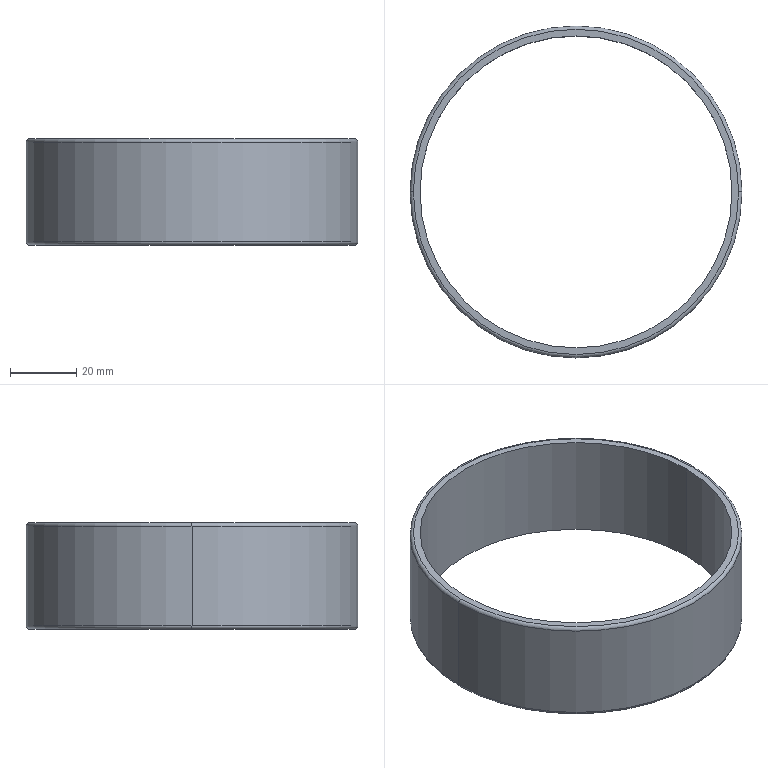Part | SolidWorks | features Extrusion 1, Fillet 1 | 1 solid | 10 faces | box 100 x 100 x 32 mm | volume 29120 mm3 | torus 4 | cylinder 4 | plane 2 | commonest cylinder face diameters 94 x2 100 x2
STEP:
#1=CARTESIAN_POINT('',(-50.,0.,31.));
#2=VERTEX_POINT('',#1);
#3=CARTESIAN_POINT('',(50.,0.,31.));
#4=VERTEX_POINT('',#3);
#5=CARTESIAN_POINT('',(0.,0.,31.));
#6=DIRECTION('',(0.,0.,-1.));
#7=DIRECTION('',(1.,0.,0.));
#8=AXIS2_PLACEMENT_3D('',#5,#6,#7);
#9=CIRCLE('',#8,50.);
#10=EDGE_CURVE('',#2,#4,#9,.T.);
#11=ORIENTED_EDGE('',*,*,#10,.F.);
#12=CARTESIAN_POINT('',(-49.,0.,32.));
#13=VERTEX_POINT('',#12);
#14=CARTESIAN_POINT('',(-49.,0.,31.));
#15=DIRECTION('',(0.,1.,0.));
#16=DIRECTION('',(-1.,0.,0.));
#17=AXIS2_PLACEMENT_3D('',#14,#15,#16);
#18=CIRCLE('',#17,1.);
#19=EDGE_CURVE('',#2,#13,#18,.T.);
#20=ORIENTED_EDGE('',*,*,#19,.T.);
#21=CARTESIAN_POINT('',(49.,0.,32.));
#22=VERTEX_POINT('',#21);
#23=CARTESIAN_POINT('',(0.,0.,32.));
#24=DIRECTION('',(0.,0.,1.));
#25=DIRECTION('',(1.,0.,0.));
#26=AXIS2_PLACEMENT_3D('',#23,#24,#25);
#27=CIRCLE('',#26,49.);
#28=EDGE_CURVE('',#22,#13,#27,.T.);
#29=ORIENTED_EDGE('',*,*,#28,.F.);
#30=CARTESIAN_POINT('',(49.,0.,31.));
#31=DIRECTION('',(0.,-1.,0.));
#32=DIRECTION('',(0.,0.,-1.));
#33=AXIS2_PLACEMENT_3D('',#30,#31,#32);
#34=CIRCLE('',#33,1.);
#35=EDGE_CURVE('',#4,#22,#34,.T.);
#36=ORIENTED_EDGE('',*,*,#35,.F.);
#37=EDGE_LOOP('',(#11,#20,#29,#36));
#38=FACE_OUTER_BOUND('',#37,.T.);
#39=CARTESIAN_POINT('',(0.,0.,31.));
#40=DIRECTION('',(0.,0.,1.));
#41=DIRECTION('',(1.,0.,0.));
#42=AXIS2_PLACEMENT_3D('',#39,#40,#41);
#43=TOROIDAL_SURFACE('',#42,49.,1.);
#44=ADVANCED_FACE('',(#38),#43,.T.);
#45=CARTESIAN_POINT('',(-49.,0.,0.));
#46=VERTEX_POINT('',#45);
#47=CARTESIAN_POINT('',(49.,0.,0.));
#48=VERTEX_POINT('',#47);
#49=CARTESIAN_POINT('',(0.,0.,0.));
#50=DIRECTION('',(0.,0.,-1.));
#51=DIRECTION('',(1.,0.,0.));
#52=AXIS2_PLACEMENT_3D('',#49,#50,#51);
#53=CIRCLE('',#52,49.);
#54=EDGE_CURVE('',#46,#48,#53,.T.);
#55=ORIENTED_EDGE('',*,*,#54,.F.);
#56=CARTESIAN_POINT('',(-50.,0.,1.));
#57=VERTEX_POINT('',#56);
#58=CARTESIAN_POINT('',(-49.,0.,1.));
#59=DIRECTION('',(0.,1.,0.));
#60=DIRECTION('',(-1.,0.,0.));
#61=AXIS2_PLACEMENT_3D('',#58,#59,#60);
#62=CIRCLE('',#61,1.);
#63=EDGE_CURVE('',#46,#57,#62,.T.);
#64=ORIENTED_EDGE('',*,*,#63,.T.);
#65=CARTESIAN_POINT('',(50.,0.,1.));
#66=VERTEX_POINT('',#65);
#67=CARTESIAN_POINT('',(0.,0.,1.));
#68=DIRECTION('',(0.,0.,1.));
#69=DIRECTION('',(1.,0.,0.));
#70=AXIS2_PLACEMENT_3D('',#67,#68,#69);
#71=CIRCLE('',#70,50.);
#72=EDGE_CURVE('',#66,#57,#71,.T.);
#73=ORIENTED_EDGE('',*,*,#72,.F.);
#74=CARTESIAN_POINT('',(49.,0.,1.));
#75=DIRECTION('',(0.,-1.,0.));
#76=DIRECTION('',(0.,0.,-1.));
#77=AXIS2_PLACEMENT_3D('',#74,#75,#76);
#78=CIRCLE('',#77,1.);
#79=EDGE_CURVE('',#48,#66,#78,.T.);
#80=ORIENTED_EDGE('',*,*,#79,.F.);
#81=EDGE_LOOP('',(#55,#64,#73,#80));
#82=FACE_OUTER_BOUND('',#81,.T.);
#83=CARTESIAN_POINT('',(0.,0.,1.));
#84=DIRECTION('',(0.,0.,1.));
#85=DIRECTION('',(1.,0.,0.));
#86=AXIS2_PLACEMENT_3D('',#83,#84,#85);
#87=TOROIDAL_SURFACE('',#86,49.,1.);
#88=ADVANCED_FACE('',(#82),#87,.T.);
#89=CARTESIAN_POINT('',(-47.,0.,32.));
#90=VERTEX_POINT('',#89);
#91=CARTESIAN_POINT('',(47.,0.,32.));
#92=VERTEX_POINT('',#91);
#93=CARTESIAN_POINT('',(0.,0.,32.));
#94=DIRECTION('',(0.,0.,1.));
#95=DIRECTION('',(1.,0.,0.));
#96=AXIS2_PLACEMENT_3D('',#93,#94,#95);
#97=CIRCLE('',#96,47.);
#98=EDGE_CURVE('',#90,#92,#97,.T.);
#99=ORIENTED_EDGE('',*,*,#98,.T.);
#100=CARTESIAN_POINT('',(47.,0.,0.));
#101=VERTEX_POINT('',#100);
#102=CARTESIAN_POINT('',(47.,0.,32.));
#103=DIRECTION('',(0.,0.,-1.));
#104=VECTOR('',#103,1000.);
#105=LINE('',#102,#104);
#106=EDGE_CURVE('',#92,#101,#105,.T.);
#107=ORIENTED_EDGE('',*,*,#106,.T.);
#108=CARTESIAN_POINT('',(-47.,0.,0.));
#109=VERTEX_POINT('',#108);
#110=CARTESIAN_POINT('',(0.,0.,0.));
#111=DIRECTION('',(0.,0.,1.));
#112=DIRECTION('',(1.,0.,0.));
#113=AXIS2_PLACEMENT_3D('',#110,#111,#112);
#114=CIRCLE('',#113,47.);
#115=EDGE_CURVE('',#109,#101,#114,.T.);
#116=ORIENTED_EDGE('',*,*,#115,.F.);
#117=CARTESIAN_POINT('',(-47.,0.,32.));
#118=DIRECTION('',(0.,0.,-1.));
#119=VECTOR('',#118,1000.);
#120=LINE('',#117,#119);
#121=EDGE_CURVE('',#90,#109,#120,.T.);
#122=ORIENTED_EDGE('',*,*,#121,.F.);
#123=EDGE_LOOP('',(#99,#107,#116,#122));
#124=FACE_OUTER_BOUND('',#123,.T.);
#125=CARTESIAN_POINT('',(0.,0.,32.));
#126=DIRECTION('',(0.,0.,-1.));
#127=DIRECTION('',(-1.,0.,0.));
#128=AXIS2_PLACEMENT_3D('',#125,#126,#127);
#129=CYLINDRICAL_SURFACE('',#128,47.);
#130=ADVANCED_FACE('',(#124),#129,.F.);
#131=ORIENTED_EDGE('',*,*,#10,.T.);
#132=CARTESIAN_POINT('',(50.,0.,32.));
#133=DIRECTION('',(0.,0.,-1.));
#134=VECTOR('',#133,1000.);
#135=LINE('',#132,#134);
#136=EDGE_CURVE('',#4,#66,#135,.T.);
#137=ORIENTED_EDGE('',*,*,#136,.T.);
#138=ORIENTED_EDGE('',*,*,#72,.T.);
#139=CARTESIAN_POINT('',(-50.,0.,32.));
#140=DIRECTION('',(0.,0.,-1.));
#141=VECTOR('',#140,1000.);
#142=LINE('',#139,#141);
#143=EDGE_CURVE('',#2,#57,#142,.T.);
#144=ORIENTED_EDGE('',*,*,#143,.F.);
#145=EDGE_LOOP('',(#131,#137,#138,#144));
#146=FACE_OUTER_BOUND('',#145,.T.);
#147=CARTESIAN_POINT('',(0.,0.,32.));
#148=DIRECTION('',(0.,0.,-1.));
#149=DIRECTION('',(-1.,0.,0.));
#150=AXIS2_PLACEMENT_3D('',#147,#148,#149);
#151=CYLINDRICAL_SURFACE('',#150,50.);
#152=ADVANCED_FACE('',(#146),#151,.T.);
#153=ORIENTED_EDGE('',*,*,#28,.T.);
#154=CARTESIAN_POINT('',(0.,0.,32.));
#155=DIRECTION('',(0.,0.,1.));
#156=DIRECTION('',(1.,0.,0.));
#157=AXIS2_PLACEMENT_3D('',#154,#155,#156);
#158=CIRCLE('',#157,49.);
#159=EDGE_CURVE('',#13,#22,#158,.T.);
#160=ORIENTED_EDGE('',*,*,#159,.T.);
#161=EDGE_LOOP('',(#153,#160));
#162=FACE_OUTER_BOUND('',#161,.T.);
#163=ORIENTED_EDGE('',*,*,#98,.F.);
#164=CARTESIAN_POINT('',(0.,0.,32.));
#165=DIRECTION('',(0.,0.,1.));
#166=DIRECTION('',(1.,0.,0.));
#167=AXIS2_PLACEMENT_3D('',#164,#165,#166);
#168=CIRCLE('',#167,47.);
#169=EDGE_CURVE('',#92,#90,#168,.T.);
#170=ORIENTED_EDGE('',*,*,#169,.F.);
#171=EDGE_LOOP('',(#163,#170));
#172=FACE_BOUND('',#171,.T.);
#173=CARTESIAN_POINT('',(0.,0.,32.));
#174=DIRECTION('',(0.,0.,1.));
#175=DIRECTION('',(1.,0.,0.));
#176=AXIS2_PLACEMENT_3D('',#173,#174,#175);
#177=PLANE('',#176);
#178=ADVANCED_FACE('',(#162,#172),#177,.T.);
#179=CARTESIAN_POINT('',(0.,0.,0.));
#180=DIRECTION('',(0.,0.,-1.));
#181=DIRECTION('',(1.,0.,0.));
#182=AXIS2_PLACEMENT_3D('',#179,#180,#181);
#183=CIRCLE('',#182,49.);
#184=EDGE_CURVE('',#48,#46,#183,.T.);
#185=ORIENTED_EDGE('',*,*,#184,.T.);
#186=ORIENTED_EDGE('',*,*,#54,.T.);
#187=EDGE_LOOP('',(#185,#186));
#188=FACE_OUTER_BOUND('',#187,.T.);
#189=ORIENTED_EDGE('',*,*,#115,.T.);
#190=CARTESIAN_POINT('',(0.,0.,0.));
#191=DIRECTION('',(0.,0.,1.));
#192=DIRECTION('',(1.,0.,0.));
#193=AXIS2_PLACEMENT_3D('',#190,#191,#192);
#194=CIRCLE('',#193,47.);
#195=EDGE_CURVE('',#101,#109,#194,.T.);
#196=ORIENTED_EDGE('',*,*,#195,.T.);
#197=EDGE_LOOP('',(#189,#196));
#198=FACE_BOUND('',#197,.T.);
#199=CARTESIAN_POINT('',(0.,0.,0.));
#200=DIRECTION('',(0.,0.,1.));
#201=DIRECTION('',(1.,0.,0.));
#202=AXIS2_PLACEMENT_3D('',#199,#200,#201);
#203=PLANE('',#202);
#204=ADVANCED_FACE('',(#188,#198),#203,.F.);
#205=ORIENTED_EDGE('',*,*,#136,.F.);
#206=CARTESIAN_POINT('',(0.,0.,31.));
#207=DIRECTION('',(0.,0.,-1.));
#208=DIRECTION('',(1.,0.,0.));
#209=AXIS2_PLACEMENT_3D('',#206,#207,#208);
#210=CIRCLE('',#209,50.);
#211=EDGE_CURVE('',#4,#2,#210,.T.);
#212=ORIENTED_EDGE('',*,*,#211,.T.);
#213=ORIENTED_EDGE('',*,*,#143,.T.);
#214=CARTESIAN_POINT('',(0.,0.,1.));
#215=DIRECTION('',(0.,0.,1.));
#216=DIRECTION('',(1.,0.,0.));
#217=AXIS2_PLACEMENT_3D('',#214,#215,#216);
#218=CIRCLE('',#217,50.);
#219=EDGE_CURVE('',#57,#66,#218,.T.);
#220=ORIENTED_EDGE('',*,*,#219,.T.);
#221=EDGE_LOOP('',(#205,#212,#213,#220));
#222=FACE_OUTER_BOUND('',#221,.T.);
#223=CARTESIAN_POINT('',(0.,0.,32.));
#224=DIRECTION('',(0.,0.,-1.));
#225=DIRECTION('',(-1.,0.,0.));
#226=AXIS2_PLACEMENT_3D('',#223,#224,#225);
#227=CYLINDRICAL_SURFACE('',#226,50.);
#228=ADVANCED_FACE('',(#222),#227,.T.);
#229=ORIENTED_EDGE('',*,*,#106,.F.);
#230=ORIENTED_EDGE('',*,*,#169,.T.);
#231=ORIENTED_EDGE('',*,*,#121,.T.);
#232=ORIENTED_EDGE('',*,*,#195,.F.);
#233=EDGE_LOOP('',(#229,#230,#231,#232));
#234=FACE_OUTER_BOUND('',#233,.T.);
#235=CARTESIAN_POINT('',(0.,0.,32.));
#236=DIRECTION('',(0.,0.,-1.));
#237=DIRECTION('',(-1.,0.,0.));
#238=AXIS2_PLACEMENT_3D('',#235,#236,#237);
#239=CYLINDRICAL_SURFACE('',#238,47.);
#240=ADVANCED_FACE('',(#234),#239,.F.);
#241=ORIENTED_EDGE('',*,*,#63,.F.);
#242=ORIENTED_EDGE('',*,*,#184,.F.);
#243=ORIENTED_EDGE('',*,*,#79,.T.);
#244=ORIENTED_EDGE('',*,*,#219,.F.);
#245=EDGE_LOOP('',(#241,#242,#243,#244));
#246=FACE_OUTER_BOUND('',#245,.T.);
#247=CARTESIAN_POINT('',(0.,0.,1.));
#248=DIRECTION('',(0.,0.,1.));
#249=DIRECTION('',(1.,0.,0.));
#250=AXIS2_PLACEMENT_3D('',#247,#248,#249);
#251=TOROIDAL_SURFACE('',#250,49.,1.);
#252=ADVANCED_FACE('',(#246),#251,.T.);
#253=ORIENTED_EDGE('',*,*,#19,.F.);
#254=ORIENTED_EDGE('',*,*,#211,.F.);
#255=ORIENTED_EDGE('',*,*,#35,.T.);
#256=ORIENTED_EDGE('',*,*,#159,.F.);
#257=EDGE_LOOP('',(#253,#254,#255,#256));
#258=FACE_OUTER_BOUND('',#257,.T.);
#259=CARTESIAN_POINT('',(0.,0.,31.));
#260=DIRECTION('',(0.,0.,1.));
#261=DIRECTION('',(1.,0.,0.));
#262=AXIS2_PLACEMENT_3D('',#259,#260,#261);
#263=TOROIDAL_SURFACE('',#262,49.,1.);
#264=ADVANCED_FACE('',(#258),#263,.T.);
#265=CLOSED_SHELL('',(#44,#88,#130,#152,#178,#204,#228,#240,#252,#264));
#266=MANIFOLD_SOLID_BREP('',#265);
#267=CARTESIAN_POINT('',(0.,0.,0.));
#268=DIRECTION('',(0.,0.,1.));
#269=DIRECTION('',(1.,0.,0.));
#270=AXIS2_PLACEMENT_3D('',#267,#268,#269);
#271=(LENGTH_UNIT()NAMED_UNIT(*)SI_UNIT(.MILLI.,.METRE.));
#272=UNCERTAINTY_MEASURE_WITH_UNIT(LENGTH_MEASURE(0.00001),#271,'','');
#273=(NAMED_UNIT(*)PLANE_ANGLE_UNIT()SI_UNIT($,.RADIAN.));
#274=(NAMED_UNIT(*)SI_UNIT($,.STERADIAN.)SOLID_ANGLE_UNIT());
#275=(GEOMETRIC_REPRESENTATION_CONTEXT(3)GLOBAL_UNCERTAINTY_ASSIGNED_CONTEXT((#272))GLOBAL_UNIT_ASSIGNED_CONTEXT((#271,#273,#274))REPRESENTATION_CONTEXT('',''));
#276=ADVANCED_BREP_SHAPE_REPRESENTATION('',(#266,#270),#275);